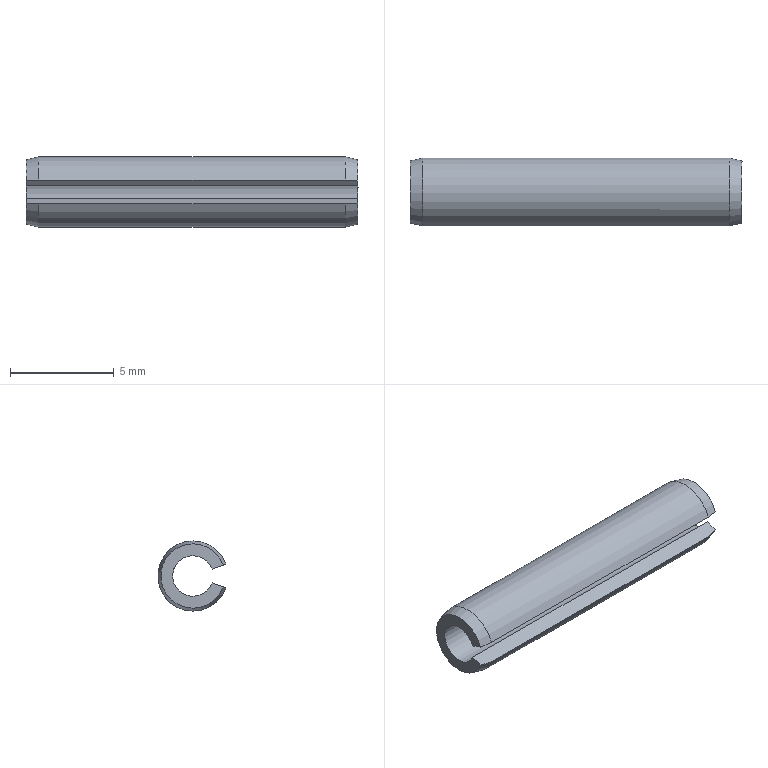Part | NX | features solid 2 | 1 solid | 8 faces | box 15.995 x 3.277 x 3.378 mm | volume 83.94 mm3 | plane 4 | cylinder 2 | cone 2 | commonest cylinder face diameters 1.956 x1 3.378 x1
STEP:
#1=CARTESIAN_POINT('',(-285.861,51.982,26.517));
#2=VERTEX_POINT('',#1);
#3=CARTESIAN_POINT('',(-285.861,51.982,27.673));
#4=VERTEX_POINT('',#3);
#5=CARTESIAN_POINT('',(-285.861,53.569,27.095));
#6=DIRECTION('',(1.,-0.00002097,-0.000000211));
#7=DIRECTION('',(-0.00001977,-0.9397,-0.342));
#8=AXIS2_PLACEMENT_3D('',#5,#6,#7);
#9=CIRCLE('',#8,1.689);
#10=EDGE_CURVE('',#2,#4,#9,.T.);
#11=ORIENTED_EDGE('',*,*,#10,.T.);
#12=CARTESIAN_POINT('',(-271.085,51.982,27.673));
#13=VERTEX_POINT('',#12);
#14=CARTESIAN_POINT('',(-285.861,51.982,27.673));
#15=DIRECTION('',(1.,-0.00002097,-0.000000211));
#16=VECTOR('',#15,1000.);
#17=LINE('',#14,#16);
#18=EDGE_CURVE('',#4,#13,#17,.T.);
#19=ORIENTED_EDGE('',*,*,#18,.T.);
#20=CARTESIAN_POINT('',(-271.085,53.569,25.406));
#21=VERTEX_POINT('',#20);
#22=CARTESIAN_POINT('',(-271.085,53.569,27.095));
#23=DIRECTION('',(1.,-0.00002097,-0.000000211));
#24=DIRECTION('',(-0.000000211,0.,-1.));
#25=AXIS2_PLACEMENT_3D('',#22,#23,#24);
#26=CIRCLE('',#25,1.689);
#27=EDGE_CURVE('',#21,#13,#26,.T.);
#28=ORIENTED_EDGE('',*,*,#27,.F.);
#29=CARTESIAN_POINT('',(-271.085,51.982,26.517));
#30=VERTEX_POINT('',#29);
#31=CARTESIAN_POINT('',(-271.085,53.569,27.095));
#32=DIRECTION('',(1.,-0.00002097,-0.000000211));
#33=DIRECTION('',(-0.00001977,-0.9397,-0.342));
#34=AXIS2_PLACEMENT_3D('',#31,#32,#33);
#35=CIRCLE('',#34,1.689);
#36=EDGE_CURVE('',#30,#21,#35,.T.);
#37=ORIENTED_EDGE('',*,*,#36,.F.);
#38=CARTESIAN_POINT('',(-271.085,51.982,26.517));
#39=DIRECTION('',(-1.,0.00002097,0.000000211));
#40=VECTOR('',#39,1000.);
#41=LINE('',#38,#40);
#42=EDGE_CURVE('',#30,#2,#41,.T.);
#43=ORIENTED_EDGE('',*,*,#42,.T.);
#44=EDGE_LOOP('',(#11,#19,#28,#37,#43));
#45=FACE_BOUND('',#44,.T.);
#46=CARTESIAN_POINT('',(-272.196,53.569,27.095));
#47=DIRECTION('',(-1.,0.00002097,0.000000211));
#48=DIRECTION('',(0.000000211,0.,1.));
#49=AXIS2_PLACEMENT_3D('',#46,#47,#48);
#50=CYLINDRICAL_SURFACE('',#49,1.689);
#51=ADVANCED_FACE('',(#45),#50,.T.);
#52=CARTESIAN_POINT('',(-286.471,52.113,26.565));
#53=VERTEX_POINT('',#52);
#54=CARTESIAN_POINT('',(-286.471,52.113,26.565));
#55=DIRECTION('',(0.9747,-0.2099,-0.0764));
#56=VECTOR('',#55,1000.);
#57=LINE('',#54,#56);
#58=EDGE_CURVE('',#53,#2,#57,.T.);
#59=ORIENTED_EDGE('',*,*,#58,.T.);
#60=ORIENTED_EDGE('',*,*,#42,.F.);
#61=CARTESIAN_POINT('',(-270.476,52.113,26.565));
#62=VERTEX_POINT('',#61);
#63=CARTESIAN_POINT('',(-271.085,51.982,26.517));
#64=DIRECTION('',(0.9747,0.2099,0.0764));
#65=VECTOR('',#64,1000.);
#66=LINE('',#63,#65);
#67=EDGE_CURVE('',#30,#62,#66,.T.);
#68=ORIENTED_EDGE('',*,*,#67,.T.);
#69=CARTESIAN_POINT('',(-270.476,52.65,26.761));
#70=VERTEX_POINT('',#69);
#71=CARTESIAN_POINT('',(-270.476,52.65,26.761));
#72=DIRECTION('',(-0.00001977,-0.9397,-0.342));
#73=VECTOR('',#72,1000.);
#74=LINE('',#71,#73);
#75=EDGE_CURVE('',#70,#62,#74,.T.);
#76=ORIENTED_EDGE('',*,*,#75,.F.);
#77=CARTESIAN_POINT('',(-286.471,52.65,26.761));
#78=VERTEX_POINT('',#77);
#79=CARTESIAN_POINT('',(-286.471,52.65,26.761));
#80=DIRECTION('',(1.,-0.00002097,-0.000000211));
#81=VECTOR('',#80,1000.);
#82=LINE('',#79,#81);
#83=EDGE_CURVE('',#78,#70,#82,.T.);
#84=ORIENTED_EDGE('',*,*,#83,.F.);
#85=CARTESIAN_POINT('',(-286.471,52.113,26.565));
#86=DIRECTION('',(0.00001977,0.9397,0.342));
#87=VECTOR('',#86,1000.);
#88=LINE('',#85,#87);
#89=EDGE_CURVE('',#53,#78,#88,.T.);
#90=ORIENTED_EDGE('',*,*,#89,.F.);
#91=EDGE_LOOP('',(#59,#60,#68,#76,#84,#90));
#92=FACE_BOUND('',#91,.T.);
#93=CARTESIAN_POINT('',(-272.196,52.65,26.761));
#94=DIRECTION('',(0.000006973,0.342,-0.9397));
#95=DIRECTION('',(0.00001977,0.9397,0.342));
#96=AXIS2_PLACEMENT_3D('',#93,#94,#95);
#97=PLANE('',#96);
#98=ADVANCED_FACE('',(#92),#97,.F.);
#99=CARTESIAN_POINT('',(-286.471,52.113,27.625));
#100=VERTEX_POINT('',#99);
#101=CARTESIAN_POINT('',(-286.471,53.569,27.095));
#102=DIRECTION('',(1.,-0.00002097,-0.000000211));
#103=DIRECTION('',(-0.00001977,-0.9397,-0.342));
#104=AXIS2_PLACEMENT_3D('',#101,#102,#103);
#105=CIRCLE('',#104,1.549);
#106=EDGE_CURVE('',#53,#100,#105,.T.);
#107=ORIENTED_EDGE('',*,*,#106,.F.);
#108=ORIENTED_EDGE('',*,*,#89,.T.);
#109=CARTESIAN_POINT('',(-286.471,53.569,26.117));
#110=VERTEX_POINT('',#109);
#111=CARTESIAN_POINT('',(-286.471,53.569,27.095));
#112=DIRECTION('',(1.,-0.00002097,-0.000000211));
#113=DIRECTION('',(-0.00001977,-0.9397,-0.342));
#114=AXIS2_PLACEMENT_3D('',#111,#112,#113);
#115=CIRCLE('',#114,0.9779);
#116=EDGE_CURVE('',#78,#110,#115,.T.);
#117=ORIENTED_EDGE('',*,*,#116,.T.);
#118=CARTESIAN_POINT('',(-286.471,52.65,27.429));
#119=VERTEX_POINT('',#118);
#120=CARTESIAN_POINT('',(-286.471,53.569,27.095));
#121=DIRECTION('',(1.,-0.00002097,-0.000000211));
#122=DIRECTION('',(-0.000000211,0.,-1.));
#123=AXIS2_PLACEMENT_3D('',#120,#121,#122);
#124=CIRCLE('',#123,0.9779);
#125=EDGE_CURVE('',#110,#119,#124,.T.);
#126=ORIENTED_EDGE('',*,*,#125,.T.);
#127=CARTESIAN_POINT('',(-286.471,52.65,27.429));
#128=DIRECTION('',(-0.00001963,-0.9397,0.342));
#129=VECTOR('',#128,1000.);
#130=LINE('',#127,#129);
#131=EDGE_CURVE('',#119,#100,#130,.T.);
#132=ORIENTED_EDGE('',*,*,#131,.T.);
#133=EDGE_LOOP('',(#107,#108,#117,#126,#132));
#134=FACE_BOUND('',#133,.T.);
#135=CARTESIAN_POINT('',(-286.471,53.569,27.095));
#136=DIRECTION('',(1.,-0.00002097,-0.000000211));
#137=DIRECTION('',(-0.000000211,0.,-1.));
#138=AXIS2_PLACEMENT_3D('',#135,#136,#137);
#139=PLANE('',#138);
#140=ADVANCED_FACE('',(#134),#139,.F.);
#141=CARTESIAN_POINT('',(-285.861,51.982,27.673));
#142=DIRECTION('',(-0.9747,0.2099,-0.0764));
#143=VECTOR('',#142,1000.);
#144=LINE('',#141,#143);
#145=EDGE_CURVE('',#4,#100,#144,.T.);
#146=ORIENTED_EDGE('',*,*,#145,.T.);
#147=ORIENTED_EDGE('',*,*,#131,.F.);
#148=CARTESIAN_POINT('',(-270.476,52.65,27.429));
#149=VERTEX_POINT('',#148);
#150=CARTESIAN_POINT('',(-270.476,52.65,27.429));
#151=DIRECTION('',(-1.,0.00002097,0.000000211));
#152=VECTOR('',#151,1000.);
#153=LINE('',#150,#152);
#154=EDGE_CURVE('',#149,#119,#153,.T.);
#155=ORIENTED_EDGE('',*,*,#154,.F.);
#156=CARTESIAN_POINT('',(-270.476,52.113,27.625));
#157=VERTEX_POINT('',#156);
#158=CARTESIAN_POINT('',(-270.476,52.113,27.625));
#159=DIRECTION('',(0.00001963,0.9397,-0.342));
#160=VECTOR('',#159,1000.);
#161=LINE('',#158,#160);
#162=EDGE_CURVE('',#157,#149,#161,.T.);
#163=ORIENTED_EDGE('',*,*,#162,.F.);
#164=CARTESIAN_POINT('',(-270.476,52.113,27.625));
#165=DIRECTION('',(-0.9747,-0.2099,0.0764));
#166=VECTOR('',#165,1000.);
#167=LINE('',#164,#166);
#168=EDGE_CURVE('',#157,#13,#167,.T.);
#169=ORIENTED_EDGE('',*,*,#168,.T.);
#170=ORIENTED_EDGE('',*,*,#18,.F.);
#171=EDGE_LOOP('',(#146,#147,#155,#163,#169,#170));
#172=FACE_BOUND('',#171,.T.);
#173=CARTESIAN_POINT('',(-272.196,51.982,27.673));
#174=DIRECTION('',(0.000007369,0.342,0.9397));
#175=DIRECTION('',(-0.00001963,-0.9397,0.342));
#176=AXIS2_PLACEMENT_3D('',#173,#174,#175);
#177=PLANE('',#176);
#178=ADVANCED_FACE('',(#172),#177,.F.);
#179=ORIENTED_EDGE('',*,*,#36,.T.);
#180=ORIENTED_EDGE('',*,*,#27,.T.);
#181=ORIENTED_EDGE('',*,*,#168,.F.);
#182=CARTESIAN_POINT('',(-270.476,53.569,25.546));
#183=VERTEX_POINT('',#182);
#184=CARTESIAN_POINT('',(-270.476,53.569,27.095));
#185=DIRECTION('',(1.,-0.00002097,-0.000000211));
#186=DIRECTION('',(-0.000000211,0.,-1.));
#187=AXIS2_PLACEMENT_3D('',#184,#185,#186);
#188=CIRCLE('',#187,1.549);
#189=EDGE_CURVE('',#183,#157,#188,.T.);
#190=ORIENTED_EDGE('',*,*,#189,.F.);
#191=CARTESIAN_POINT('',(-270.476,53.569,27.095));
#192=DIRECTION('',(1.,-0.00002097,-0.000000211));
#193=DIRECTION('',(-0.00001977,-0.9397,-0.342));
#194=AXIS2_PLACEMENT_3D('',#191,#192,#193);
#195=CIRCLE('',#194,1.549);
#196=EDGE_CURVE('',#62,#183,#195,.T.);
#197=ORIENTED_EDGE('',*,*,#196,.F.);
#198=ORIENTED_EDGE('',*,*,#67,.F.);
#199=EDGE_LOOP('',(#179,#180,#181,#190,#197,#198));
#200=FACE_BOUND('',#199,.T.);
#201=CARTESIAN_POINT('',(-270.781,53.569,27.095));
#202=DIRECTION('',(-1.,0.00002097,0.000000211));
#203=DIRECTION('',(0.000000211,0.,1.));
#204=AXIS2_PLACEMENT_3D('',#201,#202,#203);
#205=CONICAL_SURFACE('',#204,1.619,0.2253);
#206=ADVANCED_FACE('',(#200),#205,.T.);
#207=ORIENTED_EDGE('',*,*,#196,.T.);
#208=ORIENTED_EDGE('',*,*,#189,.T.);
#209=ORIENTED_EDGE('',*,*,#162,.T.);
#210=CARTESIAN_POINT('',(-270.476,53.569,26.117));
#211=VERTEX_POINT('',#210);
#212=CARTESIAN_POINT('',(-270.476,53.569,27.095));
#213=DIRECTION('',(-1.,0.00002097,0.000000211));
#214=DIRECTION('',(-0.00001963,-0.9397,0.342));
#215=AXIS2_PLACEMENT_3D('',#212,#213,#214);
#216=CIRCLE('',#215,0.9779);
#217=EDGE_CURVE('',#149,#211,#216,.T.);
#218=ORIENTED_EDGE('',*,*,#217,.T.);
#219=CARTESIAN_POINT('',(-270.476,53.569,27.095));
#220=DIRECTION('',(-1.,0.00002097,0.000000211));
#221=DIRECTION('',(-0.000000211,0.,-1.));
#222=AXIS2_PLACEMENT_3D('',#219,#220,#221);
#223=CIRCLE('',#222,0.9779);
#224=EDGE_CURVE('',#211,#70,#223,.T.);
#225=ORIENTED_EDGE('',*,*,#224,.T.);
#226=ORIENTED_EDGE('',*,*,#75,.T.);
#227=EDGE_LOOP('',(#207,#208,#209,#218,#225,#226));
#228=FACE_BOUND('',#227,.T.);
#229=CARTESIAN_POINT('',(-270.476,53.569,27.095));
#230=DIRECTION('',(1.,-0.00002097,-0.000000211));
#231=DIRECTION('',(-0.000000211,0.,-1.));
#232=AXIS2_PLACEMENT_3D('',#229,#230,#231);
#233=PLANE('',#232);
#234=ADVANCED_FACE('',(#228),#233,.T.);
#235=ORIENTED_EDGE('',*,*,#116,.F.);
#236=ORIENTED_EDGE('',*,*,#83,.T.);
#237=ORIENTED_EDGE('',*,*,#224,.F.);
#238=ORIENTED_EDGE('',*,*,#217,.F.);
#239=ORIENTED_EDGE('',*,*,#154,.T.);
#240=ORIENTED_EDGE('',*,*,#125,.F.);
#241=EDGE_LOOP('',(#235,#236,#237,#238,#239,#240));
#242=FACE_BOUND('',#241,.T.);
#243=CARTESIAN_POINT('',(-272.196,53.569,27.095));
#244=DIRECTION('',(-1.,0.00002097,0.000000211));
#245=DIRECTION('',(0.000000211,0.,1.));
#246=AXIS2_PLACEMENT_3D('',#243,#244,#245);
#247=CYLINDRICAL_SURFACE('',#246,0.9779);
#248=ADVANCED_FACE('',(#242),#247,.F.);
#249=ORIENTED_EDGE('',*,*,#106,.T.);
#250=ORIENTED_EDGE('',*,*,#145,.F.);
#251=ORIENTED_EDGE('',*,*,#10,.F.);
#252=ORIENTED_EDGE('',*,*,#58,.F.);
#253=EDGE_LOOP('',(#249,#250,#251,#252));
#254=FACE_BOUND('',#253,.T.);
#255=CARTESIAN_POINT('',(-286.166,53.569,27.095));
#256=DIRECTION('',(1.,-0.00002097,-0.000000211));
#257=DIRECTION('',(-0.000000211,0.,-1.));
#258=AXIS2_PLACEMENT_3D('',#255,#256,#257);
#259=CONICAL_SURFACE('',#258,1.619,0.2253);
#260=ADVANCED_FACE('',(#254),#259,.T.);
#261=CLOSED_SHELL('',(#51,#98,#140,#178,#206,#234,#248,#260));
#262=MANIFOLD_SOLID_BREP('',#261);
#263=(LENGTH_UNIT()NAMED_UNIT(*)SI_UNIT(.MILLI.,.METRE.));
#264=UNCERTAINTY_MEASURE_WITH_UNIT(LENGTH_MEASURE(0.00001),#263,'','');
#265=(NAMED_UNIT(*)PLANE_ANGLE_UNIT()SI_UNIT($,.RADIAN.));
#266=(NAMED_UNIT(*)SI_UNIT($,.STERADIAN.)SOLID_ANGLE_UNIT());
#267=(GEOMETRIC_REPRESENTATION_CONTEXT(3)GLOBAL_UNCERTAINTY_ASSIGNED_CONTEXT((#264))GLOBAL_UNIT_ASSIGNED_CONTEXT((#263,#265,#266))REPRESENTATION_CONTEXT('',''));
#268=ADVANCED_BREP_SHAPE_REPRESENTATION('',(#262),#267);